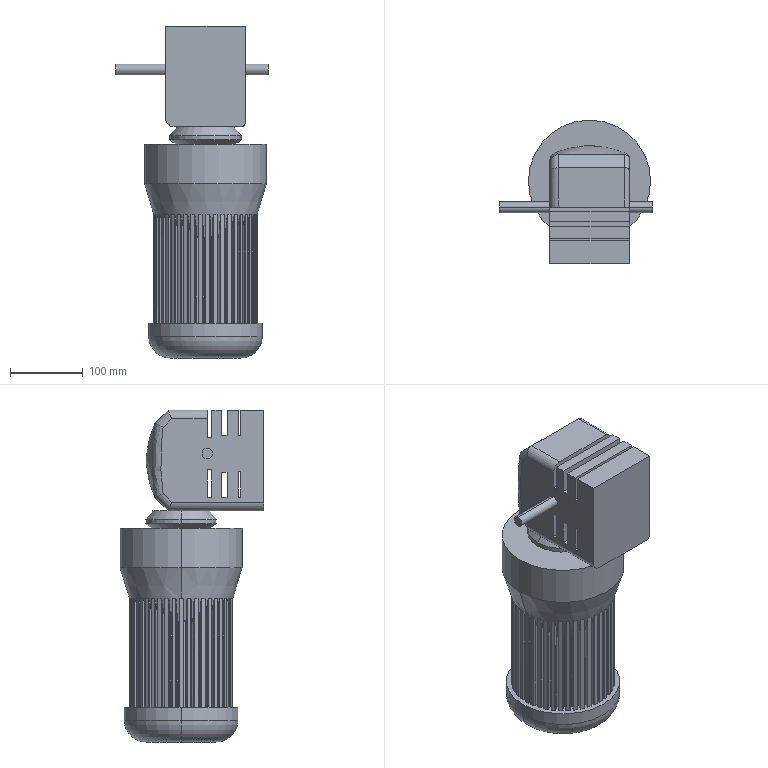Part | NX | 1 solid | 410 faces | box 210 x 198.012 x 456.821 mm | volume 7325207 mm3 | cylinder 233 | plane 166 | cone 6 | spline 3 | torus 2 | commonest cylinder face diameters 3.6 x86 5.709 x86 142.319 x43 12 x4 14.64 x4 24 x4